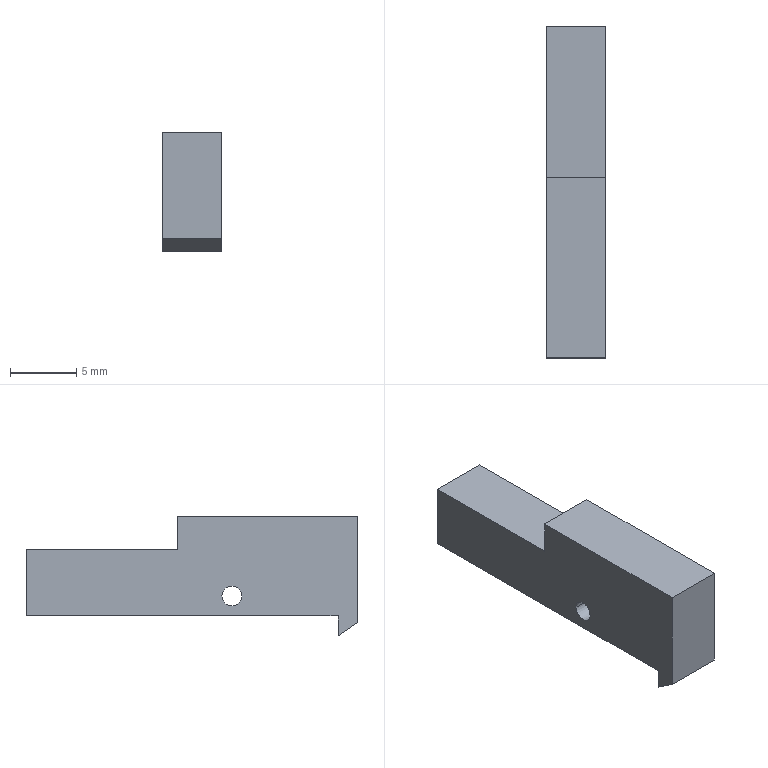Part | SolidWorks | features Cut 2, Extrusion 1, ICE 1 | 1 solid | 12 faces | box 4.5 x 25 x 9 mm | volume 714.291 mm3 | plane 10 | cylinder 2 | commonest cylinder face diameters 1.5 x2
STEP:
#1=CARTESIAN_POINT('',(-2.25,-3.75,1.5));
#2=VERTEX_POINT('',#1);
#3=CARTESIAN_POINT('',(-2.25,-2.25,1.5));
#4=VERTEX_POINT('',#3);
#5=CARTESIAN_POINT('',(-2.25,-3.,1.5));
#6=DIRECTION('',(1.,0.,0.));
#7=DIRECTION('',(0.,1.,0.));
#8=AXIS2_PLACEMENT_3D('',#5,#6,#7);
#9=CIRCLE('',#8,0.75);
#10=EDGE_CURVE('',#2,#4,#9,.T.);
#11=ORIENTED_EDGE('',*,*,#10,.F.);
#12=CARTESIAN_POINT('',(2.25,-3.75,1.5));
#13=VERTEX_POINT('',#12);
#14=CARTESIAN_POINT('',(-2.25,-3.75,1.5));
#15=DIRECTION('',(1.,0.,0.));
#16=VECTOR('',#15,1000.);
#17=LINE('',#14,#16);
#18=EDGE_CURVE('',#2,#13,#17,.T.);
#19=ORIENTED_EDGE('',*,*,#18,.T.);
#20=CARTESIAN_POINT('',(2.25,-2.25,1.5));
#21=VERTEX_POINT('',#20);
#22=CARTESIAN_POINT('',(2.25,-3.,1.5));
#23=DIRECTION('',(1.,0.,0.));
#24=DIRECTION('',(0.,1.,0.));
#25=AXIS2_PLACEMENT_3D('',#22,#23,#24);
#26=CIRCLE('',#25,0.75);
#27=EDGE_CURVE('',#13,#21,#26,.T.);
#28=ORIENTED_EDGE('',*,*,#27,.T.);
#29=CARTESIAN_POINT('',(-2.25,-2.25,1.5));
#30=DIRECTION('',(1.,0.,0.));
#31=VECTOR('',#30,1000.);
#32=LINE('',#29,#31);
#33=EDGE_CURVE('',#4,#21,#32,.T.);
#34=ORIENTED_EDGE('',*,*,#33,.F.);
#35=EDGE_LOOP('',(#11,#19,#28,#34));
#36=FACE_OUTER_BOUND('',#35,.T.);
#37=CARTESIAN_POINT('',(-2.25,-3.,1.5));
#38=DIRECTION('',(1.,0.,0.));
#39=DIRECTION('',(0.,1.,0.));
#40=AXIS2_PLACEMENT_3D('',#37,#38,#39);
#41=CYLINDRICAL_SURFACE('',#40,0.75);
#42=ADVANCED_FACE('',(#36),#41,.F.);
#43=CARTESIAN_POINT('',(-2.25,-11.,0.));
#44=VERTEX_POINT('',#43);
#45=CARTESIAN_POINT('',(2.25,-11.,0.));
#46=VERTEX_POINT('',#45);
#47=CARTESIAN_POINT('',(-4.371,-11.,0.));
#48=DIRECTION('',(1.,0.,0.));
#49=VECTOR('',#48,1000.);
#50=LINE('',#47,#49);
#51=EDGE_CURVE('',#44,#46,#50,.T.);
#52=ORIENTED_EDGE('',*,*,#51,.F.);
#53=CARTESIAN_POINT('',(-2.25,12.5,0.));
#54=VERTEX_POINT('',#53);
#55=CARTESIAN_POINT('',(-2.25,12.5,0.));
#56=DIRECTION('',(0.,-1.,0.));
#57=VECTOR('',#56,1000.);
#58=LINE('',#55,#57);
#59=EDGE_CURVE('',#54,#44,#58,.T.);
#60=ORIENTED_EDGE('',*,*,#59,.F.);
#61=CARTESIAN_POINT('',(2.25,12.5,0.));
#62=VERTEX_POINT('',#61);
#63=CARTESIAN_POINT('',(-2.25,12.5,0.));
#64=DIRECTION('',(-1.,0.,0.));
#65=VECTOR('',#64,1000.);
#66=LINE('',#63,#65);
#67=EDGE_CURVE('',#62,#54,#66,.T.);
#68=ORIENTED_EDGE('',*,*,#67,.F.);
#69=CARTESIAN_POINT('',(2.25,12.5,0.));
#70=DIRECTION('',(0.,1.,0.));
#71=VECTOR('',#70,1000.);
#72=LINE('',#69,#71);
#73=EDGE_CURVE('',#46,#62,#72,.T.);
#74=ORIENTED_EDGE('',*,*,#73,.F.);
#75=EDGE_LOOP('',(#52,#60,#68,#74));
#76=FACE_OUTER_BOUND('',#75,.T.);
#77=CARTESIAN_POINT('',(0.,0.,0.));
#78=DIRECTION('',(0.,0.,1.));
#79=DIRECTION('',(1.,0.,0.));
#80=AXIS2_PLACEMENT_3D('',#77,#78,#79);
#81=PLANE('',#80);
#82=ADVANCED_FACE('',(#76),#81,.F.);
#83=CARTESIAN_POINT('',(2.25,-3.,1.5));
#84=DIRECTION('',(1.,0.,0.));
#85=DIRECTION('',(0.,1.,0.));
#86=AXIS2_PLACEMENT_3D('',#83,#84,#85);
#87=CIRCLE('',#86,0.75);
#88=EDGE_CURVE('',#21,#13,#87,.T.);
#89=ORIENTED_EDGE('',*,*,#88,.F.);
#90=ORIENTED_EDGE('',*,*,#27,.F.);
#91=EDGE_LOOP('',(#89,#90));
#92=FACE_BOUND('',#91,.T.);
#93=CARTESIAN_POINT('',(2.25,12.5,5.));
#94=VERTEX_POINT('',#93);
#95=CARTESIAN_POINT('',(2.25,1.099,5.));
#96=VERTEX_POINT('',#95);
#97=CARTESIAN_POINT('',(2.25,12.5,5.));
#98=DIRECTION('',(0.,-1.,0.));
#99=VECTOR('',#98,1000.);
#100=LINE('',#97,#99);
#101=EDGE_CURVE('',#94,#96,#100,.T.);
#102=ORIENTED_EDGE('',*,*,#101,.T.);
#103=CARTESIAN_POINT('',(2.25,1.099,7.5));
#104=VERTEX_POINT('',#103);
#105=CARTESIAN_POINT('',(2.25,1.099,7.5));
#106=DIRECTION('',(0.,0.,1.));
#107=VECTOR('',#106,1000.);
#108=LINE('',#105,#107);
#109=EDGE_CURVE('',#96,#104,#108,.T.);
#110=ORIENTED_EDGE('',*,*,#109,.T.);
#111=CARTESIAN_POINT('',(2.25,-12.5,7.5));
#112=VERTEX_POINT('',#111);
#113=CARTESIAN_POINT('',(2.25,12.5,7.5));
#114=DIRECTION('',(0.,1.,0.));
#115=VECTOR('',#114,1000.);
#116=LINE('',#113,#115);
#117=EDGE_CURVE('',#112,#104,#116,.T.);
#118=ORIENTED_EDGE('',*,*,#117,.F.);
#119=CARTESIAN_POINT('',(2.25,-12.5,-0.5));
#120=VERTEX_POINT('',#119);
#121=CARTESIAN_POINT('',(2.25,-12.5,7.5));
#122=DIRECTION('',(0.,0.,-1.));
#123=VECTOR('',#122,1000.);
#124=LINE('',#121,#123);
#125=EDGE_CURVE('',#112,#120,#124,.T.);
#126=ORIENTED_EDGE('',*,*,#125,.T.);
#127=CARTESIAN_POINT('',(2.25,-11.,-1.5));
#128=VERTEX_POINT('',#127);
#129=CARTESIAN_POINT('',(2.25,-12.5,-0.5));
#130=DIRECTION('',(0.,0.8321,-0.5547));
#131=VECTOR('',#130,1000.);
#132=LINE('',#129,#131);
#133=EDGE_CURVE('',#120,#128,#132,.T.);
#134=ORIENTED_EDGE('',*,*,#133,.T.);
#135=CARTESIAN_POINT('',(2.25,-11.,-1.5));
#136=DIRECTION('',(0.,0.,1.));
#137=VECTOR('',#136,1000.);
#138=LINE('',#135,#137);
#139=EDGE_CURVE('',#128,#46,#138,.T.);
#140=ORIENTED_EDGE('',*,*,#139,.T.);
#141=ORIENTED_EDGE('',*,*,#73,.T.);
#142=CARTESIAN_POINT('',(2.25,12.5,7.5));
#143=DIRECTION('',(0.,0.,-1.));
#144=VECTOR('',#143,1000.);
#145=LINE('',#142,#144);
#146=EDGE_CURVE('',#94,#62,#145,.T.);
#147=ORIENTED_EDGE('',*,*,#146,.F.);
#148=EDGE_LOOP('',(#102,#110,#118,#126,#134,#140,#141,#147));
#149=FACE_OUTER_BOUND('',#148,.T.);
#150=CARTESIAN_POINT('',(2.25,12.5,7.5));
#151=DIRECTION('',(-1.,0.,0.));
#152=DIRECTION('',(0.,-1.,0.));
#153=AXIS2_PLACEMENT_3D('',#150,#151,#152);
#154=PLANE('',#153);
#155=ADVANCED_FACE('',(#92,#149),#154,.F.);
#156=CARTESIAN_POINT('',(-2.25,12.5,5.));
#157=VERTEX_POINT('',#156);
#158=CARTESIAN_POINT('',(-2.25,12.5,7.5));
#159=DIRECTION('',(0.,0.,-1.));
#160=VECTOR('',#159,1000.);
#161=LINE('',#158,#160);
#162=EDGE_CURVE('',#157,#54,#161,.T.);
#163=ORIENTED_EDGE('',*,*,#162,.F.);
#164=CARTESIAN_POINT('',(2.25,12.5,5.));
#165=DIRECTION('',(-1.,0.,0.));
#166=VECTOR('',#165,1000.);
#167=LINE('',#164,#166);
#168=EDGE_CURVE('',#94,#157,#167,.T.);
#169=ORIENTED_EDGE('',*,*,#168,.F.);
#170=ORIENTED_EDGE('',*,*,#146,.T.);
#171=ORIENTED_EDGE('',*,*,#67,.T.);
#172=EDGE_LOOP('',(#163,#169,#170,#171));
#173=FACE_OUTER_BOUND('',#172,.T.);
#174=CARTESIAN_POINT('',(-2.25,12.5,7.5));
#175=DIRECTION('',(0.,-1.,0.));
#176=DIRECTION('',(0.,0.,-1.));
#177=AXIS2_PLACEMENT_3D('',#174,#175,#176);
#178=PLANE('',#177);
#179=ADVANCED_FACE('',(#173),#178,.F.);
#180=CARTESIAN_POINT('',(-2.25,-3.,1.5));
#181=DIRECTION('',(1.,0.,0.));
#182=DIRECTION('',(0.,1.,0.));
#183=AXIS2_PLACEMENT_3D('',#180,#181,#182);
#184=CIRCLE('',#183,0.75);
#185=EDGE_CURVE('',#4,#2,#184,.T.);
#186=ORIENTED_EDGE('',*,*,#185,.T.);
#187=ORIENTED_EDGE('',*,*,#10,.T.);
#188=EDGE_LOOP('',(#186,#187));
#189=FACE_BOUND('',#188,.T.);
#190=CARTESIAN_POINT('',(-2.25,1.099,7.5));
#191=VERTEX_POINT('',#190);
#192=CARTESIAN_POINT('',(-2.25,-12.5,7.5));
#193=VERTEX_POINT('',#192);
#194=CARTESIAN_POINT('',(-2.25,12.5,7.5));
#195=DIRECTION('',(0.,-1.,0.));
#196=VECTOR('',#195,1000.);
#197=LINE('',#194,#196);
#198=EDGE_CURVE('',#191,#193,#197,.T.);
#199=ORIENTED_EDGE('',*,*,#198,.F.);
#200=CARTESIAN_POINT('',(-2.25,1.099,5.));
#201=VERTEX_POINT('',#200);
#202=CARTESIAN_POINT('',(-2.25,1.099,7.5));
#203=DIRECTION('',(0.,0.,1.));
#204=VECTOR('',#203,1000.);
#205=LINE('',#202,#204);
#206=EDGE_CURVE('',#201,#191,#205,.T.);
#207=ORIENTED_EDGE('',*,*,#206,.F.);
#208=CARTESIAN_POINT('',(-2.25,12.5,5.));
#209=DIRECTION('',(0.,-1.,0.));
#210=VECTOR('',#209,1000.);
#211=LINE('',#208,#210);
#212=EDGE_CURVE('',#157,#201,#211,.T.);
#213=ORIENTED_EDGE('',*,*,#212,.F.);
#214=ORIENTED_EDGE('',*,*,#162,.T.);
#215=ORIENTED_EDGE('',*,*,#59,.T.);
#216=CARTESIAN_POINT('',(-2.25,-11.,-1.5));
#217=VERTEX_POINT('',#216);
#218=CARTESIAN_POINT('',(-2.25,-11.,-1.5));
#219=DIRECTION('',(0.,0.,-1.));
#220=VECTOR('',#219,1000.);
#221=LINE('',#218,#220);
#222=EDGE_CURVE('',#44,#217,#221,.T.);
#223=ORIENTED_EDGE('',*,*,#222,.T.);
#224=CARTESIAN_POINT('',(-2.25,-12.5,-0.5));
#225=VERTEX_POINT('',#224);
#226=CARTESIAN_POINT('',(-2.25,-12.5,-0.5));
#227=DIRECTION('',(0.,-0.8321,0.5547));
#228=VECTOR('',#227,1000.);
#229=LINE('',#226,#228);
#230=EDGE_CURVE('',#217,#225,#229,.T.);
#231=ORIENTED_EDGE('',*,*,#230,.T.);
#232=CARTESIAN_POINT('',(-2.25,-12.5,7.5));
#233=DIRECTION('',(0.,0.,-1.));
#234=VECTOR('',#233,1000.);
#235=LINE('',#232,#234);
#236=EDGE_CURVE('',#193,#225,#235,.T.);
#237=ORIENTED_EDGE('',*,*,#236,.F.);
#238=EDGE_LOOP('',(#199,#207,#213,#214,#215,#223,#231,#237));
#239=FACE_OUTER_BOUND('',#238,.T.);
#240=CARTESIAN_POINT('',(-2.25,12.5,7.5));
#241=DIRECTION('',(1.,0.,0.));
#242=DIRECTION('',(0.,1.,0.));
#243=AXIS2_PLACEMENT_3D('',#240,#241,#242);
#244=PLANE('',#243);
#245=ADVANCED_FACE('',(#189,#239),#244,.F.);
#246=ORIENTED_EDGE('',*,*,#236,.T.);
#247=CARTESIAN_POINT('',(-4.371,-12.5,-0.5));
#248=DIRECTION('',(1.,0.,0.));
#249=VECTOR('',#248,1000.);
#250=LINE('',#247,#249);
#251=EDGE_CURVE('',#225,#120,#250,.T.);
#252=ORIENTED_EDGE('',*,*,#251,.T.);
#253=ORIENTED_EDGE('',*,*,#125,.F.);
#254=CARTESIAN_POINT('',(-2.25,-12.5,7.5));
#255=DIRECTION('',(1.,0.,0.));
#256=VECTOR('',#255,1000.);
#257=LINE('',#254,#256);
#258=EDGE_CURVE('',#193,#112,#257,.T.);
#259=ORIENTED_EDGE('',*,*,#258,.F.);
#260=EDGE_LOOP('',(#246,#252,#253,#259));
#261=FACE_OUTER_BOUND('',#260,.T.);
#262=CARTESIAN_POINT('',(-2.25,-12.5,7.5));
#263=DIRECTION('',(0.,1.,0.));
#264=DIRECTION('',(0.,0.,1.));
#265=AXIS2_PLACEMENT_3D('',#262,#263,#264);
#266=PLANE('',#265);
#267=ADVANCED_FACE('',(#261),#266,.F.);
#268=CARTESIAN_POINT('',(2.25,1.099,7.5));
#269=DIRECTION('',(-1.,0.,0.));
#270=VECTOR('',#269,1000.);
#271=LINE('',#268,#270);
#272=EDGE_CURVE('',#104,#191,#271,.T.);
#273=ORIENTED_EDGE('',*,*,#272,.T.);
#274=ORIENTED_EDGE('',*,*,#198,.T.);
#275=ORIENTED_EDGE('',*,*,#258,.T.);
#276=ORIENTED_EDGE('',*,*,#117,.T.);
#277=EDGE_LOOP('',(#273,#274,#275,#276));
#278=FACE_OUTER_BOUND('',#277,.T.);
#279=CARTESIAN_POINT('',(0.,0.,7.5));
#280=DIRECTION('',(0.,0.,1.));
#281=DIRECTION('',(1.,0.,0.));
#282=AXIS2_PLACEMENT_3D('',#279,#280,#281);
#283=PLANE('',#282);
#284=ADVANCED_FACE('',(#278),#283,.T.);
#285=ORIENTED_EDGE('',*,*,#222,.F.);
#286=ORIENTED_EDGE('',*,*,#51,.T.);
#287=ORIENTED_EDGE('',*,*,#139,.F.);
#288=CARTESIAN_POINT('',(-4.371,-11.,-1.5));
#289=DIRECTION('',(1.,0.,0.));
#290=VECTOR('',#289,1000.);
#291=LINE('',#288,#290);
#292=EDGE_CURVE('',#217,#128,#291,.T.);
#293=ORIENTED_EDGE('',*,*,#292,.F.);
#294=EDGE_LOOP('',(#285,#286,#287,#293));
#295=FACE_OUTER_BOUND('',#294,.T.);
#296=CARTESIAN_POINT('',(-4.371,-11.,-1.5));
#297=DIRECTION('',(0.,1.,0.));
#298=DIRECTION('',(-1.,0.,0.));
#299=AXIS2_PLACEMENT_3D('',#296,#297,#298);
#300=PLANE('',#299);
#301=ADVANCED_FACE('',(#295),#300,.T.);
#302=ORIENTED_EDGE('',*,*,#230,.F.);
#303=ORIENTED_EDGE('',*,*,#292,.T.);
#304=ORIENTED_EDGE('',*,*,#133,.F.);
#305=ORIENTED_EDGE('',*,*,#251,.F.);
#306=EDGE_LOOP('',(#302,#303,#304,#305));
#307=FACE_OUTER_BOUND('',#306,.T.);
#308=CARTESIAN_POINT('',(-4.371,-12.5,-0.5));
#309=DIRECTION('',(0.,-0.5547,-0.8321));
#310=DIRECTION('',(0.,0.8321,-0.5547));
#311=AXIS2_PLACEMENT_3D('',#308,#309,#310);
#312=PLANE('',#311);
#313=ADVANCED_FACE('',(#307),#312,.T.);
#314=ORIENTED_EDGE('',*,*,#18,.F.);
#315=ORIENTED_EDGE('',*,*,#185,.F.);
#316=ORIENTED_EDGE('',*,*,#33,.T.);
#317=ORIENTED_EDGE('',*,*,#88,.T.);
#318=EDGE_LOOP('',(#314,#315,#316,#317));
#319=FACE_OUTER_BOUND('',#318,.T.);
#320=CARTESIAN_POINT('',(-2.25,-3.,1.5));
#321=DIRECTION('',(1.,0.,0.));
#322=DIRECTION('',(0.,1.,0.));
#323=AXIS2_PLACEMENT_3D('',#320,#321,#322);
#324=CYLINDRICAL_SURFACE('',#323,0.75);
#325=ADVANCED_FACE('',(#319),#324,.F.);
#326=ORIENTED_EDGE('',*,*,#206,.T.);
#327=ORIENTED_EDGE('',*,*,#272,.F.);
#328=ORIENTED_EDGE('',*,*,#109,.F.);
#329=CARTESIAN_POINT('',(2.25,1.099,5.));
#330=DIRECTION('',(-1.,0.,0.));
#331=VECTOR('',#330,1000.);
#332=LINE('',#329,#331);
#333=EDGE_CURVE('',#96,#201,#332,.T.);
#334=ORIENTED_EDGE('',*,*,#333,.T.);
#335=EDGE_LOOP('',(#326,#327,#328,#334));
#336=FACE_OUTER_BOUND('',#335,.T.);
#337=CARTESIAN_POINT('',(2.25,1.099,7.5));
#338=DIRECTION('',(0.,-1.,0.));
#339=DIRECTION('',(1.,0.,0.));
#340=AXIS2_PLACEMENT_3D('',#337,#338,#339);
#341=PLANE('',#340);
#342=ADVANCED_FACE('',(#336),#341,.F.);
#343=ORIENTED_EDGE('',*,*,#212,.T.);
#344=ORIENTED_EDGE('',*,*,#333,.F.);
#345=ORIENTED_EDGE('',*,*,#101,.F.);
#346=ORIENTED_EDGE('',*,*,#168,.T.);
#347=EDGE_LOOP('',(#343,#344,#345,#346));
#348=FACE_OUTER_BOUND('',#347,.T.);
#349=CARTESIAN_POINT('',(2.25,12.5,5.));
#350=DIRECTION('',(0.,0.,-1.));
#351=DIRECTION('',(0.,1.,0.));
#352=AXIS2_PLACEMENT_3D('',#349,#350,#351);
#353=PLANE('',#352);
#354=ADVANCED_FACE('',(#348),#353,.F.);
#355=CLOSED_SHELL('',(#42,#82,#155,#179,#245,#267,#284,#301,#313,#325,#342,#354));
#356=MANIFOLD_SOLID_BREP('',#355);
#357=CARTESIAN_POINT('',(0.,0.,0.));
#358=DIRECTION('',(0.,0.,1.));
#359=DIRECTION('',(1.,0.,0.));
#360=AXIS2_PLACEMENT_3D('',#357,#358,#359);
#361=(LENGTH_UNIT()NAMED_UNIT(*)SI_UNIT(.MILLI.,.METRE.));
#362=UNCERTAINTY_MEASURE_WITH_UNIT(LENGTH_MEASURE(0.00001),#361,'','');
#363=(NAMED_UNIT(*)PLANE_ANGLE_UNIT()SI_UNIT($,.RADIAN.));
#364=(NAMED_UNIT(*)SI_UNIT($,.STERADIAN.)SOLID_ANGLE_UNIT());
#365=(GEOMETRIC_REPRESENTATION_CONTEXT(3)GLOBAL_UNCERTAINTY_ASSIGNED_CONTEXT((#362))GLOBAL_UNIT_ASSIGNED_CONTEXT((#361,#363,#364))REPRESENTATION_CONTEXT('',''));
#366=ADVANCED_BREP_SHAPE_REPRESENTATION('',(#356,#360),#365);